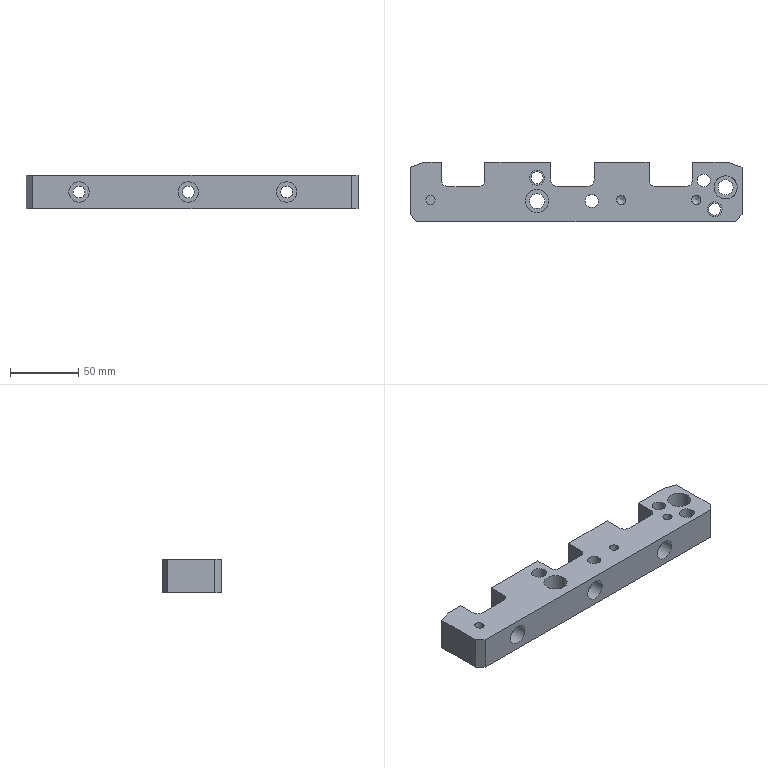Part | STEP file | 1_id1510_x_t | 1 solid | 63 faces | box 243 x 43.296 x 24.5 mm | volume 189026 mm3 | plane 32 | cylinder 27 | cone 4 | commonest cylinder face diameters 9.525 x4 11 x4 6.75 x3 8.7 x3 15 x3 8 x2